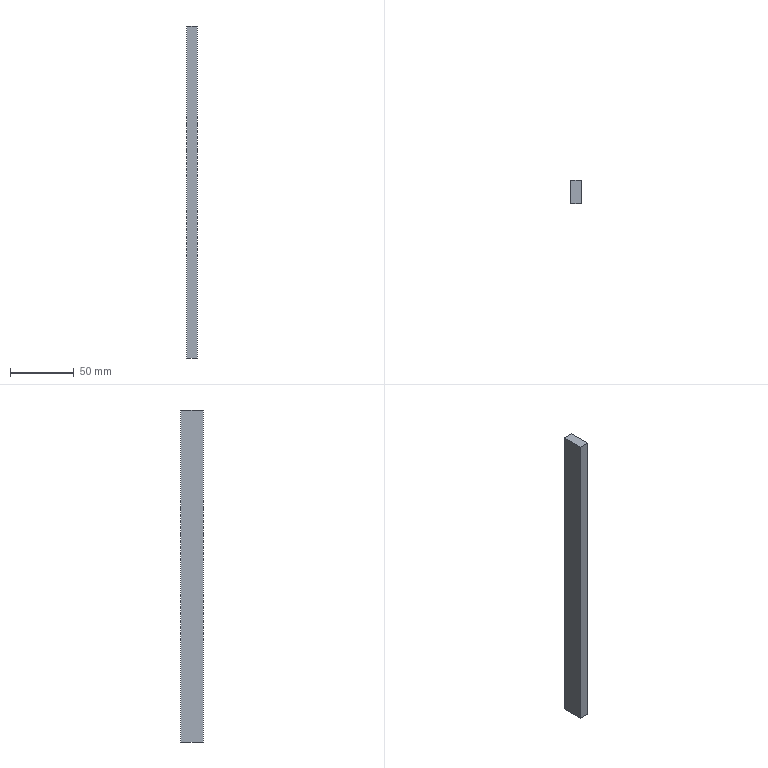Part | SolidWorks | features Extrusion 1 | 1 solid | 6 faces | box 8 x 18 x 260 mm | volume 37440 mm3 | plane 6
STEP:
#1=CARTESIAN_POINT('',(-4.,9.,130.));
#2=VERTEX_POINT('',#1);
#3=CARTESIAN_POINT('',(-4.,-9.,130.));
#4=VERTEX_POINT('',#3);
#5=CARTESIAN_POINT('',(-4.,9.,130.));
#6=DIRECTION('',(0.,-1.,0.));
#7=VECTOR('',#6,1000.);
#8=LINE('',#5,#7);
#9=EDGE_CURVE('',#2,#4,#8,.T.);
#10=ORIENTED_EDGE('',*,*,#9,.F.);
#11=CARTESIAN_POINT('',(-4.,9.,-130.));
#12=VERTEX_POINT('',#11);
#13=CARTESIAN_POINT('',(-4.,9.,-130.));
#14=DIRECTION('',(0.,0.,1.));
#15=VECTOR('',#14,1000.);
#16=LINE('',#13,#15);
#17=EDGE_CURVE('',#12,#2,#16,.T.);
#18=ORIENTED_EDGE('',*,*,#17,.F.);
#19=CARTESIAN_POINT('',(-4.,-9.,-130.));
#20=VERTEX_POINT('',#19);
#21=CARTESIAN_POINT('',(-4.,9.,-130.));
#22=DIRECTION('',(0.,-1.,0.));
#23=VECTOR('',#22,1000.);
#24=LINE('',#21,#23);
#25=EDGE_CURVE('',#12,#20,#24,.T.);
#26=ORIENTED_EDGE('',*,*,#25,.T.);
#27=CARTESIAN_POINT('',(-4.,-9.,-130.));
#28=DIRECTION('',(0.,0.,1.));
#29=VECTOR('',#28,1000.);
#30=LINE('',#27,#29);
#31=EDGE_CURVE('',#20,#4,#30,.T.);
#32=ORIENTED_EDGE('',*,*,#31,.T.);
#33=EDGE_LOOP('',(#10,#18,#26,#32));
#34=FACE_OUTER_BOUND('',#33,.T.);
#35=CARTESIAN_POINT('',(-4.,9.,-130.));
#36=DIRECTION('',(-1.,0.,0.));
#37=DIRECTION('',(0.,0.,1.));
#38=AXIS2_PLACEMENT_3D('',#35,#36,#37);
#39=PLANE('',#38);
#40=ADVANCED_FACE('',(#34),#39,.T.);
#41=CARTESIAN_POINT('',(4.,9.,130.));
#42=VERTEX_POINT('',#41);
#43=CARTESIAN_POINT('',(4.,9.,130.));
#44=DIRECTION('',(-1.,0.,0.));
#45=VECTOR('',#44,1000.);
#46=LINE('',#43,#45);
#47=EDGE_CURVE('',#42,#2,#46,.T.);
#48=ORIENTED_EDGE('',*,*,#47,.F.);
#49=CARTESIAN_POINT('',(4.,9.,-130.));
#50=VERTEX_POINT('',#49);
#51=CARTESIAN_POINT('',(4.,9.,-130.));
#52=DIRECTION('',(0.,0.,1.));
#53=VECTOR('',#52,1000.);
#54=LINE('',#51,#53);
#55=EDGE_CURVE('',#50,#42,#54,.T.);
#56=ORIENTED_EDGE('',*,*,#55,.F.);
#57=CARTESIAN_POINT('',(4.,9.,-130.));
#58=DIRECTION('',(-1.,0.,0.));
#59=VECTOR('',#58,1000.);
#60=LINE('',#57,#59);
#61=EDGE_CURVE('',#50,#12,#60,.T.);
#62=ORIENTED_EDGE('',*,*,#61,.T.);
#63=ORIENTED_EDGE('',*,*,#17,.T.);
#64=EDGE_LOOP('',(#48,#56,#62,#63));
#65=FACE_OUTER_BOUND('',#64,.T.);
#66=CARTESIAN_POINT('',(4.,9.,-130.));
#67=DIRECTION('',(0.,1.,0.));
#68=DIRECTION('',(0.,0.,1.));
#69=AXIS2_PLACEMENT_3D('',#66,#67,#68);
#70=PLANE('',#69);
#71=ADVANCED_FACE('',(#65),#70,.T.);
#72=CARTESIAN_POINT('',(4.,-9.,130.));
#73=VERTEX_POINT('',#72);
#74=CARTESIAN_POINT('',(4.,-9.,130.));
#75=DIRECTION('',(0.,1.,0.));
#76=VECTOR('',#75,1000.);
#77=LINE('',#74,#76);
#78=EDGE_CURVE('',#73,#42,#77,.T.);
#79=ORIENTED_EDGE('',*,*,#78,.F.);
#80=CARTESIAN_POINT('',(4.,-9.,-130.));
#81=VERTEX_POINT('',#80);
#82=CARTESIAN_POINT('',(4.,-9.,-130.));
#83=DIRECTION('',(0.,0.,1.));
#84=VECTOR('',#83,1000.);
#85=LINE('',#82,#84);
#86=EDGE_CURVE('',#81,#73,#85,.T.);
#87=ORIENTED_EDGE('',*,*,#86,.F.);
#88=CARTESIAN_POINT('',(4.,-9.,-130.));
#89=DIRECTION('',(0.,1.,0.));
#90=VECTOR('',#89,1000.);
#91=LINE('',#88,#90);
#92=EDGE_CURVE('',#81,#50,#91,.T.);
#93=ORIENTED_EDGE('',*,*,#92,.T.);
#94=ORIENTED_EDGE('',*,*,#55,.T.);
#95=EDGE_LOOP('',(#79,#87,#93,#94));
#96=FACE_OUTER_BOUND('',#95,.T.);
#97=CARTESIAN_POINT('',(4.,-9.,-130.));
#98=DIRECTION('',(1.,0.,0.));
#99=DIRECTION('',(0.,0.,-1.));
#100=AXIS2_PLACEMENT_3D('',#97,#98,#99);
#101=PLANE('',#100);
#102=ADVANCED_FACE('',(#96),#101,.T.);
#103=CARTESIAN_POINT('',(-4.,-9.,130.));
#104=DIRECTION('',(1.,0.,0.));
#105=VECTOR('',#104,1000.);
#106=LINE('',#103,#105);
#107=EDGE_CURVE('',#4,#73,#106,.T.);
#108=ORIENTED_EDGE('',*,*,#107,.F.);
#109=ORIENTED_EDGE('',*,*,#31,.F.);
#110=CARTESIAN_POINT('',(-4.,-9.,-130.));
#111=DIRECTION('',(1.,0.,0.));
#112=VECTOR('',#111,1000.);
#113=LINE('',#110,#112);
#114=EDGE_CURVE('',#20,#81,#113,.T.);
#115=ORIENTED_EDGE('',*,*,#114,.T.);
#116=ORIENTED_EDGE('',*,*,#86,.T.);
#117=EDGE_LOOP('',(#108,#109,#115,#116));
#118=FACE_OUTER_BOUND('',#117,.T.);
#119=CARTESIAN_POINT('',(-4.,-9.,-130.));
#120=DIRECTION('',(0.,-1.,0.));
#121=DIRECTION('',(0.,0.,-1.));
#122=AXIS2_PLACEMENT_3D('',#119,#120,#121);
#123=PLANE('',#122);
#124=ADVANCED_FACE('',(#118),#123,.T.);
#125=ORIENTED_EDGE('',*,*,#25,.F.);
#126=ORIENTED_EDGE('',*,*,#61,.F.);
#127=ORIENTED_EDGE('',*,*,#92,.F.);
#128=ORIENTED_EDGE('',*,*,#114,.F.);
#129=EDGE_LOOP('',(#125,#126,#127,#128));
#130=FACE_OUTER_BOUND('',#129,.T.);
#131=CARTESIAN_POINT('',(0.,0.,-130.));
#132=DIRECTION('',(0.,0.,1.));
#133=DIRECTION('',(1.,0.,0.));
#134=AXIS2_PLACEMENT_3D('',#131,#132,#133);
#135=PLANE('',#134);
#136=ADVANCED_FACE('',(#130),#135,.F.);
#137=ORIENTED_EDGE('',*,*,#9,.T.);
#138=ORIENTED_EDGE('',*,*,#107,.T.);
#139=ORIENTED_EDGE('',*,*,#78,.T.);
#140=ORIENTED_EDGE('',*,*,#47,.T.);
#141=EDGE_LOOP('',(#137,#138,#139,#140));
#142=FACE_OUTER_BOUND('',#141,.T.);
#143=CARTESIAN_POINT('',(0.,0.,130.));
#144=DIRECTION('',(0.,0.,1.));
#145=DIRECTION('',(1.,0.,0.));
#146=AXIS2_PLACEMENT_3D('',#143,#144,#145);
#147=PLANE('',#146);
#148=ADVANCED_FACE('',(#142),#147,.T.);
#149=CLOSED_SHELL('',(#40,#71,#102,#124,#136,#148));
#150=MANIFOLD_SOLID_BREP('',#149);
#151=CARTESIAN_POINT('',(0.,0.,0.));
#152=DIRECTION('',(0.,0.,1.));
#153=DIRECTION('',(1.,0.,0.));
#154=AXIS2_PLACEMENT_3D('',#151,#152,#153);
#155=(LENGTH_UNIT()NAMED_UNIT(*)SI_UNIT(.MILLI.,.METRE.));
#156=UNCERTAINTY_MEASURE_WITH_UNIT(LENGTH_MEASURE(0.00001),#155,'','');
#157=(NAMED_UNIT(*)PLANE_ANGLE_UNIT()SI_UNIT($,.RADIAN.));
#158=(NAMED_UNIT(*)SI_UNIT($,.STERADIAN.)SOLID_ANGLE_UNIT());
#159=(GEOMETRIC_REPRESENTATION_CONTEXT(3)GLOBAL_UNCERTAINTY_ASSIGNED_CONTEXT((#156))GLOBAL_UNIT_ASSIGNED_CONTEXT((#155,#157,#158))REPRESENTATION_CONTEXT('',''));
#160=ADVANCED_BREP_SHAPE_REPRESENTATION('',(#150,#154),#159);